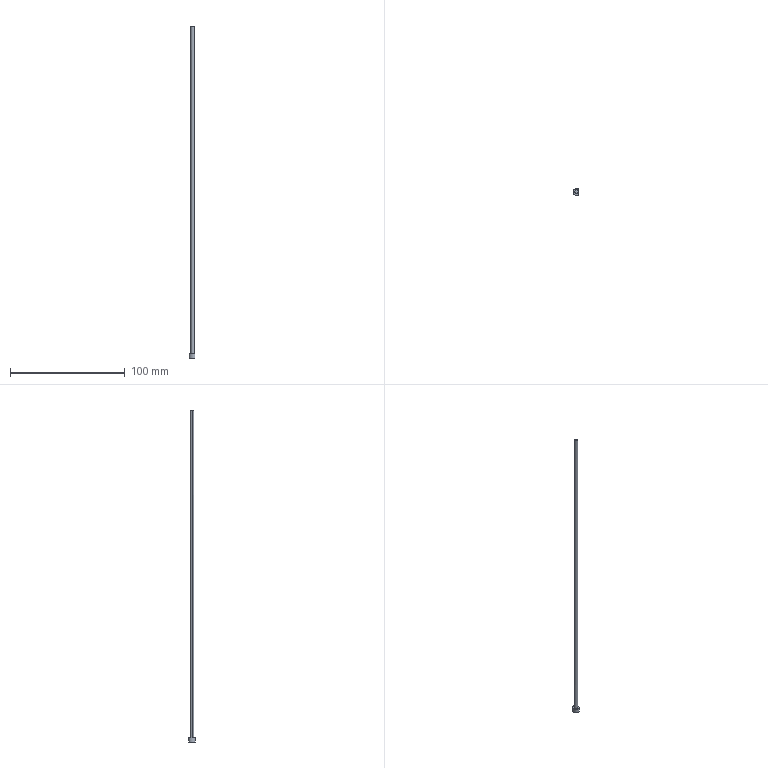Part | Creo | 1 solid | 7 faces | box 5 x 6 x 288.968 mm | volume 2114 mm3 | plane 4 | cylinder 3 | commonest cylinder face diameters 3 x2 6 x1
STEP:
#1=CARTESIAN_POINT('',(76.5,63.5,-292.));
#2=VERTEX_POINT('',#1);
#3=CARTESIAN_POINT('',(73.5,63.5,-292.));
#4=VERTEX_POINT('',#3);
#5=CARTESIAN_POINT('',(75.,63.5,-292.));
#6=DIRECTION('',(0.,0.,-1.));
#7=DIRECTION('',(1.,0.,0.));
#8=AXIS2_PLACEMENT_3D('',#5,#6,#7);
#9=CIRCLE('',#8,1.5);
#10=EDGE_CURVE('',#2,#4,#9,.T.);
#11=ORIENTED_EDGE('',*,*,#10,.T.);
#12=CARTESIAN_POINT('',(73.5,63.5,-7.032));
#13=VERTEX_POINT('',#12);
#14=CARTESIAN_POINT('',(73.5,63.5,-7.032));
#15=DIRECTION('',(0.,0.000000001,-1.));
#16=VECTOR('',#15,284.968);
#17=LINE('',#14,#16);
#18=EDGE_CURVE('',#13,#4,#17,.T.);
#19=ORIENTED_EDGE('',*,*,#18,.F.);
#20=CARTESIAN_POINT('',(76.5,63.5,-7.189));
#21=VERTEX_POINT('',#20);
#22=CARTESIAN_POINT('',(76.5,63.5,-7.189));
#23=CARTESIAN_POINT('',(76.5,63.146,-7.189));
#24=CARTESIAN_POINT('',(76.277,62.523,-7.178));
#25=CARTESIAN_POINT('',(75.554,62.064,-7.14));
#26=CARTESIAN_POINT('',(75.,61.968,-7.111));
#27=CARTESIAN_POINT('',(74.446,62.064,-7.082));
#28=CARTESIAN_POINT('',(73.723,62.523,-7.044));
#29=CARTESIAN_POINT('',(73.5,63.146,-7.032));
#30=CARTESIAN_POINT('',(73.5,63.5,-7.032));
#31=B_SPLINE_CURVE_WITH_KNOTS('',3,(#22,#23,#24,#25,#26,#27,#28,#29,#30),.UNSPECIFIED.,.F.,.F.,(4,1,1,1,1,1,4),(0.,0.25,0.375,0.5,0.625,0.75,1.),.UNSPECIFIED.);
#32=EDGE_CURVE('',#21,#13,#31,.T.);
#33=ORIENTED_EDGE('',*,*,#32,.F.);
#34=CARTESIAN_POINT('',(76.5,63.5,-7.189));
#35=DIRECTION('',(0.,-0.000000001,-1.));
#36=VECTOR('',#35,284.811);
#37=LINE('',#34,#36);
#38=EDGE_CURVE('',#21,#2,#37,.T.);
#39=ORIENTED_EDGE('',*,*,#38,.T.);
#40=EDGE_LOOP('',(#11,#19,#33,#39));
#41=FACE_OUTER_BOUND('',#40,.F.);
#42=CARTESIAN_POINT('',(75.,63.5,-5.));
#43=DIRECTION('',(0.,0.,-1.));
#44=DIRECTION('',(1.,0.,0.));
#45=AXIS2_PLACEMENT_3D('',#42,#43,#44);
#46=CYLINDRICAL_SURFACE('',#45,1.5);
#47=ADVANCED_FACE('',(#41),#46,.T.);
#48=CARTESIAN_POINT('',(77.,61.264,-292.));
#49=VERTEX_POINT('',#48);
#50=CARTESIAN_POINT('',(77.,65.736,-292.));
#51=VERTEX_POINT('',#50);
#52=CARTESIAN_POINT('',(77.,61.264,-292.));
#53=DIRECTION('',(0.,1.,0.));
#54=VECTOR('',#53,4.472);
#55=LINE('',#52,#54);
#56=EDGE_CURVE('',#49,#51,#55,.T.);
#57=ORIENTED_EDGE('',*,*,#56,.F.);
#58=CARTESIAN_POINT('',(72.,63.5,-292.));
#59=VERTEX_POINT('',#58);
#60=CARTESIAN_POINT('',(75.,63.5,-292.));
#61=DIRECTION('',(0.,0.,1.));
#62=DIRECTION('',(-1.,0.,0.));
#63=AXIS2_PLACEMENT_3D('',#60,#61,#62);
#64=CIRCLE('',#63,3.);
#65=EDGE_CURVE('',#59,#49,#64,.T.);
#66=ORIENTED_EDGE('',*,*,#65,.F.);
#67=CARTESIAN_POINT('',(75.,63.5,-292.));
#68=DIRECTION('',(0.,0.,1.));
#69=DIRECTION('',(0.6667,0.7454,0.));
#70=AXIS2_PLACEMENT_3D('',#67,#68,#69);
#71=CIRCLE('',#70,3.);
#72=EDGE_CURVE('',#51,#59,#71,.T.);
#73=ORIENTED_EDGE('',*,*,#72,.F.);
#74=EDGE_LOOP('',(#57,#66,#73));
#75=FACE_OUTER_BOUND('',#74,.F.);
#76=ORIENTED_EDGE('',*,*,#10,.F.);
#77=CARTESIAN_POINT('',(75.,63.5,-292.));
#78=DIRECTION('',(0.,0.,-1.));
#79=DIRECTION('',(-1.,0.,0.));
#80=AXIS2_PLACEMENT_3D('',#77,#78,#79);
#81=CIRCLE('',#80,1.5);
#82=EDGE_CURVE('',#4,#2,#81,.T.);
#83=ORIENTED_EDGE('',*,*,#82,.F.);
#84=EDGE_LOOP('',(#76,#83));
#85=FACE_BOUND('',#84,.F.);
#86=CARTESIAN_POINT('',(75.,63.5,-292.));
#87=DIRECTION('',(0.,0.,1.));
#88=DIRECTION('',(-1.,0.,0.));
#89=AXIS2_PLACEMENT_3D('',#86,#87,#88);
#90=PLANE('',#89);
#91=ADVANCED_FACE('',(#75,#85),#90,.T.);
#92=CARTESIAN_POINT('',(77.,61.264,-296.));
#93=VERTEX_POINT('',#92);
#94=CARTESIAN_POINT('',(77.,61.264,-296.));
#95=DIRECTION('',(0.,0.,1.));
#96=VECTOR('',#95,4.);
#97=LINE('',#94,#96);
#98=EDGE_CURVE('',#93,#49,#97,.T.);
#99=ORIENTED_EDGE('',*,*,#98,.T.);
#100=ORIENTED_EDGE('',*,*,#56,.T.);
#101=CARTESIAN_POINT('',(77.,65.736,-296.));
#102=VERTEX_POINT('',#101);
#103=CARTESIAN_POINT('',(77.,65.736,-292.));
#104=DIRECTION('',(0.,0.,-1.));
#105=VECTOR('',#104,4.);
#106=LINE('',#103,#105);
#107=EDGE_CURVE('',#51,#102,#106,.T.);
#108=ORIENTED_EDGE('',*,*,#107,.T.);
#109=CARTESIAN_POINT('',(77.,61.264,-296.));
#110=DIRECTION('',(0.,1.,0.));
#111=VECTOR('',#110,4.472);
#112=LINE('',#109,#111);
#113=EDGE_CURVE('',#93,#102,#112,.T.);
#114=ORIENTED_EDGE('',*,*,#113,.F.);
#115=EDGE_LOOP('',(#99,#100,#108,#114));
#116=FACE_OUTER_BOUND('',#115,.F.);
#117=CARTESIAN_POINT('',(77.,63.5,-296.));
#118=DIRECTION('',(-1.,0.,0.));
#119=DIRECTION('',(0.,0.,1.));
#120=AXIS2_PLACEMENT_3D('',#117,#118,#119);
#121=PLANE('',#120);
#122=ADVANCED_FACE('',(#116),#121,.F.);
#123=ORIENTED_EDGE('',*,*,#98,.F.);
#124=CARTESIAN_POINT('',(72.,63.5,-296.));
#125=VERTEX_POINT('',#124);
#126=CARTESIAN_POINT('',(75.,63.5,-296.));
#127=DIRECTION('',(0.,0.,-1.));
#128=DIRECTION('',(0.6667,-0.7454,0.));
#129=AXIS2_PLACEMENT_3D('',#126,#127,#128);
#130=CIRCLE('',#129,3.);
#131=EDGE_CURVE('',#93,#125,#130,.T.);
#132=ORIENTED_EDGE('',*,*,#131,.T.);
#133=CARTESIAN_POINT('',(75.,63.5,-296.));
#134=DIRECTION('',(0.,0.,-1.));
#135=DIRECTION('',(-1.,0.,0.));
#136=AXIS2_PLACEMENT_3D('',#133,#134,#135);
#137=CIRCLE('',#136,3.);
#138=EDGE_CURVE('',#125,#102,#137,.T.);
#139=ORIENTED_EDGE('',*,*,#138,.T.);
#140=ORIENTED_EDGE('',*,*,#107,.F.);
#141=ORIENTED_EDGE('',*,*,#72,.T.);
#142=ORIENTED_EDGE('',*,*,#65,.T.);
#143=EDGE_LOOP('',(#123,#132,#139,#140,#141,#142));
#144=FACE_OUTER_BOUND('',#143,.F.);
#145=CARTESIAN_POINT('',(75.,63.5,-296.));
#146=DIRECTION('',(0.,0.,1.));
#147=DIRECTION('',(-1.,0.,0.));
#148=AXIS2_PLACEMENT_3D('',#145,#146,#147);
#149=CYLINDRICAL_SURFACE('',#148,3.);
#150=ADVANCED_FACE('',(#144),#149,.T.);
#151=ORIENTED_EDGE('',*,*,#131,.F.);
#152=ORIENTED_EDGE('',*,*,#113,.T.);
#153=ORIENTED_EDGE('',*,*,#138,.F.);
#154=EDGE_LOOP('',(#151,#152,#153));
#155=FACE_OUTER_BOUND('',#154,.F.);
#156=CARTESIAN_POINT('',(7.7,2.155,-296.));
#157=DIRECTION('',(0.,0.,1.));
#158=DIRECTION('',(0.,-1.,0.));
#159=AXIS2_PLACEMENT_3D('',#156,#157,#158);
#160=PLANE('',#159);
#161=ADVANCED_FACE('',(#155),#160,.F.);
#162=ORIENTED_EDGE('',*,*,#82,.T.);
#163=ORIENTED_EDGE('',*,*,#38,.F.);
#164=CARTESIAN_POINT('',(73.5,63.5,-7.032));
#165=CARTESIAN_POINT('',(73.5,63.854,-7.032));
#166=CARTESIAN_POINT('',(73.723,64.477,-7.044));
#167=CARTESIAN_POINT('',(74.446,64.936,-7.082));
#168=CARTESIAN_POINT('',(75.,65.032,-7.111));
#169=CARTESIAN_POINT('',(75.554,64.936,-7.14));
#170=CARTESIAN_POINT('',(76.277,64.477,-7.178));
#171=CARTESIAN_POINT('',(76.5,63.854,-7.189));
#172=CARTESIAN_POINT('',(76.5,63.5,-7.189));
#173=B_SPLINE_CURVE_WITH_KNOTS('',3,(#164,#165,#166,#167,#168,#169,#170,#171,#172),.UNSPECIFIED.,.F.,.F.,(4,1,1,1,1,1,4),(0.,0.25,0.375,0.5,0.625,0.75,1.),.UNSPECIFIED.);
#174=EDGE_CURVE('',#13,#21,#173,.T.);
#175=ORIENTED_EDGE('',*,*,#174,.F.);
#176=ORIENTED_EDGE('',*,*,#18,.T.);
#177=EDGE_LOOP('',(#162,#163,#175,#176));
#178=FACE_OUTER_BOUND('',#177,.F.);
#179=CARTESIAN_POINT('',(75.,63.5,-5.));
#180=DIRECTION('',(0.,0.,-1.));
#181=DIRECTION('',(1.,0.,0.));
#182=AXIS2_PLACEMENT_3D('',#179,#180,#181);
#183=CYLINDRICAL_SURFACE('',#182,1.5);
#184=ADVANCED_FACE('',(#178),#183,.T.);
#185=ORIENTED_EDGE('',*,*,#174,.T.);
#186=ORIENTED_EDGE('',*,*,#32,.T.);
#187=EDGE_LOOP('',(#185,#186));
#188=FACE_OUTER_BOUND('',#187,.F.);
#189=CARTESIAN_POINT('',(308.361,351.75,-19.338));
#190=DIRECTION('',(0.05232,0.000000032,0.9986));
#191=DIRECTION('',(-0.000000001,1.,-0.000000032));
#192=AXIS2_PLACEMENT_3D('',#189,#190,#191);
#193=PLANE('',#192);
#194=ADVANCED_FACE('',(#188),#193,.T.);
#195=CLOSED_SHELL('',(#47,#91,#122,#150,#161,#184,#194));
#196=MANIFOLD_SOLID_BREP('',#195);
#197=(LENGTH_UNIT()NAMED_UNIT(*)SI_UNIT(.MILLI.,.METRE.));
#198=UNCERTAINTY_MEASURE_WITH_UNIT(LENGTH_MEASURE(0.02891),#197,'','');
#199=(NAMED_UNIT(*)PLANE_ANGLE_UNIT()SI_UNIT($,.RADIAN.));
#200=PLANE_ANGLE_MEASURE_WITH_UNIT(PLANE_ANGLE_MEASURE(0.01745),#199);
#201=(CONVERSION_BASED_UNIT('DEGREE',#200)NAMED_UNIT(*)PLANE_ANGLE_UNIT());
#202=(NAMED_UNIT(*)SI_UNIT($,.STERADIAN.)SOLID_ANGLE_UNIT());
#203=(GEOMETRIC_REPRESENTATION_CONTEXT(3)GLOBAL_UNCERTAINTY_ASSIGNED_CONTEXT((#198))GLOBAL_UNIT_ASSIGNED_CONTEXT((#197,#201,#202))REPRESENTATION_CONTEXT('',''));
#204=ADVANCED_BREP_SHAPE_REPRESENTATION('',(#196),#203);